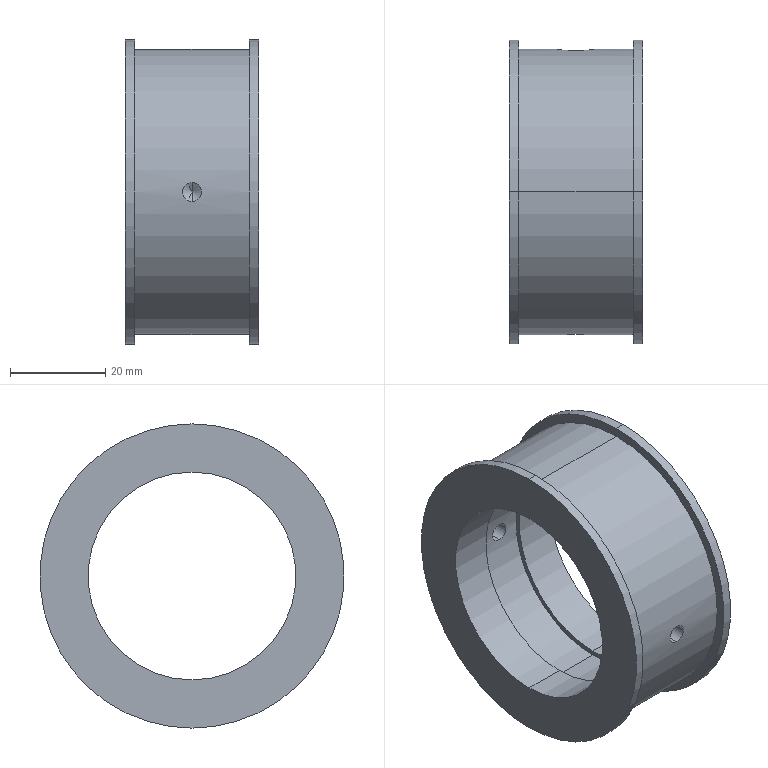Part | SolidWorks | features HoleWzd 3, Fillet 2, Revolution 1 | 1 solid | 31 faces | box 28 x 64 x 64 mm | volume 37136 mm3 | cylinder 18 | plane 7 | torus 2 | spline 2 | cone 2 | commonest cylinder face diameters 4 x4 43.7 x4 64 x4 7.5 x2 45.7 x2 60 x2
STEP:
#1=CARTESIAN_POINT('',(5.61,28.8,3.75));
#2=VERTEX_POINT('',#1);
#3=CARTESIAN_POINT('',(5.61,28.8,-3.75));
#4=VERTEX_POINT('',#3);
#5=CARTESIAN_POINT('',(5.61,28.8,0.));
#6=DIRECTION('',(0.,-1.,0.));
#7=DIRECTION('',(0.,0.,-1.));
#8=AXIS2_PLACEMENT_3D('',#5,#6,#7);
#9=CIRCLE('',#8,3.75);
#10=EDGE_CURVE('',#2,#4,#9,.T.);
#11=ORIENTED_EDGE('',*,*,#10,.F.);
#12=CARTESIAN_POINT('',(5.61,28.5,3.45));
#13=VERTEX_POINT('',#12);
#14=CARTESIAN_POINT('',(5.61,28.8,3.45));
#15=DIRECTION('',(1.,0.,0.));
#16=DIRECTION('',(0.,0.,-1.));
#17=AXIS2_PLACEMENT_3D('',#14,#15,#16);
#18=CIRCLE('',#17,0.3);
#19=EDGE_CURVE('',#2,#13,#18,.T.);
#20=ORIENTED_EDGE('',*,*,#19,.T.);
#21=CARTESIAN_POINT('',(5.61,28.5,-3.45));
#22=VERTEX_POINT('',#21);
#23=CARTESIAN_POINT('',(5.61,28.5,0.));
#24=DIRECTION('',(0.,1.,0.));
#25=DIRECTION('',(0.,0.,-1.));
#26=AXIS2_PLACEMENT_3D('',#23,#24,#25);
#27=CIRCLE('',#26,3.45);
#28=EDGE_CURVE('',#22,#13,#27,.T.);
#29=ORIENTED_EDGE('',*,*,#28,.F.);
#30=CARTESIAN_POINT('',(5.61,28.8,-3.45));
#31=DIRECTION('',(-1.,0.,0.));
#32=DIRECTION('',(0.,0.,1.));
#33=AXIS2_PLACEMENT_3D('',#30,#31,#32);
#34=CIRCLE('',#33,0.3);
#35=EDGE_CURVE('',#4,#22,#34,.T.);
#36=ORIENTED_EDGE('',*,*,#35,.F.);
#37=EDGE_LOOP('',(#11,#20,#29,#36));
#38=FACE_OUTER_BOUND('',#37,.T.);
#39=CARTESIAN_POINT('',(5.61,28.8,0.));
#40=DIRECTION('',(0.,-1.,0.));
#41=DIRECTION('',(0.,0.,-1.));
#42=AXIS2_PLACEMENT_3D('',#39,#40,#41);
#43=TOROIDAL_SURFACE('',#42,3.45,0.3);
#44=ADVANCED_FACE('',(#38),#43,.F.);
#45=CARTESIAN_POINT('',(4.758,29.551,-3.652));
#46=VERTEX_POINT('',#45);
#47=CARTESIAN_POINT('',(5.61,29.537,3.75));
#48=VERTEX_POINT('',#47);
#49=CARTESIAN_POINT('',(4.758,29.551,-3.652));
#50=CARTESIAN_POINT('',(4.535,29.558,-3.6));
#51=CARTESIAN_POINT('',(4.316,29.568,-3.527));
#52=CARTESIAN_POINT('',(3.899,29.591,-3.345));
#53=CARTESIAN_POINT('',(3.701,29.605,-3.236));
#54=CARTESIAN_POINT('',(3.325,29.634,-2.982));
#55=CARTESIAN_POINT('',(3.146,29.65,-2.836));
#56=CARTESIAN_POINT('',(2.822,29.682,-2.518));
#57=CARTESIAN_POINT('',(2.676,29.698,-2.346));
#58=CARTESIAN_POINT('',(2.414,29.728,-1.974));
#59=CARTESIAN_POINT('',(2.299,29.742,-1.774));
#60=CARTESIAN_POINT('',(2.109,29.766,-1.363));
#61=CARTESIAN_POINT('',(2.033,29.776,-1.149));
#62=CARTESIAN_POINT('',(1.92,29.792,-0.7059));
#63=CARTESIAN_POINT('',(1.884,29.797,-0.479));
#64=CARTESIAN_POINT('',(1.854,29.801,-0.02683));
#65=CARTESIAN_POINT('',(1.859,29.8,0.2003));
#66=CARTESIAN_POINT('',(1.911,29.793,0.6567));
#67=CARTESIAN_POINT('',(1.958,29.786,0.8794));
#68=CARTESIAN_POINT('',(2.09,29.769,1.312));
#69=CARTESIAN_POINT('',(2.177,29.757,1.524));
#70=CARTESIAN_POINT('',(2.387,29.731,1.93));
#71=CARTESIAN_POINT('',(2.509,29.717,2.121));
#72=CARTESIAN_POINT('',(2.787,29.686,2.478));
#73=CARTESIAN_POINT('',(2.944,29.67,2.647));
#74=CARTESIAN_POINT('',(3.284,29.638,2.95));
#75=CARTESIAN_POINT('',(3.466,29.623,3.084));
#76=CARTESIAN_POINT('',(3.853,29.594,3.32));
#77=CARTESIAN_POINT('',(4.06,29.581,3.422));
#78=CARTESIAN_POINT('',(4.485,29.56,3.584));
#79=CARTESIAN_POINT('',(4.703,29.552,3.646));
#80=CARTESIAN_POINT('',(5.15,29.54,3.729));
#81=CARTESIAN_POINT('',(5.38,29.537,3.75));
#82=CARTESIAN_POINT('',(5.61,29.537,3.75));
#83=B_SPLINE_CURVE_WITH_KNOTS('',3,(#49,#50,#51,#52,#53,#54,#55,#56,#57,#58,#59,#60,#61,#62,#63,#64,#65,#66,#67,#68,#69,#70,#71,#72,#73,#74,#75,#76,#77,#78,#79,#80,#81,#82),.UNSPECIFIED.,.F.,.F.,(4,2,2,2,2,2,2,2,2,2,2,2,2,2,2,2,4),(0.01269,0.01337,0.01406,0.01474,0.01543,0.01611,0.0168,0.01748,0.01817,0.01885,0.01954,0.02022,0.02091,0.02159,0.02228,0.02296,0.02365),.UNSPECIFIED.);
#84=EDGE_CURVE('',#46,#48,#83,.T.);
#85=ORIENTED_EDGE('',*,*,#84,.F.);
#86=CARTESIAN_POINT('',(4.712,29.749,-3.872));
#87=VERTEX_POINT('',#86);
#88=CARTESIAN_POINT('',(4.712,29.551,-3.847));
#89=DIRECTION('',(-0.9734,0.02959,0.2273));
#90=DIRECTION('',(0.2274,0.,0.9738));
#91=AXIS2_PLACEMENT_3D('',#88,#89,#90);
#92=CIRCLE('',#91,0.2);
#93=EDGE_CURVE('',#46,#87,#92,.T.);
#94=ORIENTED_EDGE('',*,*,#93,.T.);
#95=CARTESIAN_POINT('',(6.509,29.749,3.872));
#96=VERTEX_POINT('',#95);
#97=CARTESIAN_POINT('',(6.509,29.749,3.872));
#98=CARTESIAN_POINT('',(6.254,29.741,3.932));
#99=CARTESIAN_POINT('',(5.996,29.737,3.966));
#100=CARTESIAN_POINT('',(5.474,29.734,3.983));
#101=CARTESIAN_POINT('',(5.21,29.737,3.965));
#102=CARTESIAN_POINT('',(4.698,29.748,3.878));
#103=CARTESIAN_POINT('',(4.449,29.757,3.81));
#104=CARTESIAN_POINT('',(3.965,29.78,3.624));
#105=CARTESIAN_POINT('',(3.729,29.795,3.506));
#106=CARTESIAN_POINT('',(3.293,29.826,3.231));
#107=CARTESIAN_POINT('',(3.089,29.843,3.072));
#108=CARTESIAN_POINT('',(2.711,29.878,2.714));
#109=CARTESIAN_POINT('',(2.541,29.895,2.517));
#110=CARTESIAN_POINT('',(2.244,29.927,2.096));
#111=CARTESIAN_POINT('',(2.114,29.943,1.869));
#112=CARTESIAN_POINT('',(1.902,29.969,1.394));
#113=CARTESIAN_POINT('',(1.82,29.979,1.149));
#114=CARTESIAN_POINT('',(1.704,29.994,0.6447));
#115=CARTESIAN_POINT('',(1.67,29.999,0.3829));
#116=CARTESIAN_POINT('',(1.654,30.001,-0.135));
#117=CARTESIAN_POINT('',(1.671,29.999,-0.3927));
#118=CARTESIAN_POINT('',(1.755,29.987,-0.9056));
#119=CARTESIAN_POINT('',(1.823,29.979,-1.16));
#120=CARTESIAN_POINT('',(2.004,29.956,-1.643));
#121=CARTESIAN_POINT('',(2.118,29.942,-1.876));
#122=CARTESIAN_POINT('',(2.392,29.911,-2.321));
#123=CARTESIAN_POINT('',(2.549,29.894,-2.526));
#124=CARTESIAN_POINT('',(2.9,29.86,-2.904));
#125=CARTESIAN_POINT('',(3.096,29.842,-3.078));
#126=CARTESIAN_POINT('',(3.516,29.809,-3.382));
#127=CARTESIAN_POINT('',(3.739,29.794,-3.512));
#128=CARTESIAN_POINT('',(4.21,29.768,-3.727));
#129=CARTESIAN_POINT('',(4.459,29.757,-3.813));
#130=CARTESIAN_POINT('',(4.712,29.749,-3.872));
#131=B_SPLINE_CURVE_WITH_KNOTS('',3,(#97,#98,#99,#100,#101,#102,#103,#104,#105,#106,#107,#108,#109,#110,#111,#112,#113,#114,#115,#116,#117,#118,#119,#120,#121,#122,#123,#124,#125,#126,#127,#128,#129,#130),.UNSPECIFIED.,.F.,.F.,(4,2,2,2,2,2,2,2,2,2,2,2,2,2,2,2,4),(0.02421,0.025,0.02578,0.02657,0.02735,0.02814,0.02892,0.02971,0.03049,0.03128,0.03206,0.03285,0.03363,0.03442,0.0352,0.03599,0.03677),.UNSPECIFIED.);
#132=EDGE_CURVE('',#96,#87,#131,.T.);
#133=ORIENTED_EDGE('',*,*,#132,.F.);
#134=CARTESIAN_POINT('',(6.463,29.551,3.652));
#135=VERTEX_POINT('',#134);
#136=CARTESIAN_POINT('',(6.509,29.551,3.846));
#137=DIRECTION('',(0.9734,0.02959,-0.2273));
#138=DIRECTION('',(-0.2274,0.,-0.9738));
#139=AXIS2_PLACEMENT_3D('',#136,#137,#138);
#140=CIRCLE('',#139,0.2);
#141=EDGE_CURVE('',#135,#96,#140,.T.);
#142=ORIENTED_EDGE('',*,*,#141,.F.);
#143=CARTESIAN_POINT('',(5.61,29.537,3.75));
#144=CARTESIAN_POINT('',(5.754,29.537,3.75));
#145=CARTESIAN_POINT('',(6.041,29.539,3.733));
#146=CARTESIAN_POINT('',(6.323,29.546,3.684));
#147=CARTESIAN_POINT('',(6.463,29.551,3.652));
#148=B_SPLINE_CURVE_WITH_KNOTS('',3,(#143,#144,#145,#146,#147),.UNSPECIFIED.,.F.,.F.,(4,1,4),(0.,0.0004293,0.0008586),.UNSPECIFIED.);
#149=EDGE_CURVE('',#48,#135,#148,.T.);
#150=ORIENTED_EDGE('',*,*,#149,.F.);
#151=EDGE_LOOP('',(#85,#94,#133,#142,#150));
#152=FACE_OUTER_BOUND('',#151,.T.);
#153=CARTESIAN_POINT('',(6.463,29.551,3.652));
#154=CARTESIAN_POINT('',(6.457,29.778,3.653));
#155=CARTESIAN_POINT('',(6.509,29.749,3.872));
#156=CARTESIAN_POINT('',(6.222,29.543,3.708));
#157=CARTESIAN_POINT('',(6.216,29.771,3.709));
#158=CARTESIAN_POINT('',(6.254,29.741,3.932));
#159=CARTESIAN_POINT('',(5.979,29.538,3.74));
#160=CARTESIAN_POINT('',(5.976,29.767,3.74));
#161=CARTESIAN_POINT('',(5.998,29.737,3.966));
#162=CARTESIAN_POINT('',(5.49,29.536,3.756));
#163=CARTESIAN_POINT('',(5.491,29.765,3.756));
#164=CARTESIAN_POINT('',(5.484,29.734,3.983));
#165=CARTESIAN_POINT('',(5.241,29.539,3.74));
#166=CARTESIAN_POINT('',(5.245,29.767,3.74));
#167=CARTESIAN_POINT('',(5.222,29.737,3.966));
#168=CARTESIAN_POINT('',(4.756,29.55,3.66));
#169=CARTESIAN_POINT('',(4.763,29.777,3.661));
#170=CARTESIAN_POINT('',(4.71,29.748,3.881));
#171=CARTESIAN_POINT('',(4.52,29.558,3.596));
#172=CARTESIAN_POINT('',(4.529,29.784,3.599));
#173=CARTESIAN_POINT('',(4.462,29.757,3.814));
#174=CARTESIAN_POINT('',(4.061,29.581,3.424));
#175=CARTESIAN_POINT('',(4.072,29.804,3.429));
#176=CARTESIAN_POINT('',(3.978,29.78,3.631));
#177=CARTESIAN_POINT('',(3.837,29.595,3.313));
#178=CARTESIAN_POINT('',(3.849,29.817,3.32));
#179=CARTESIAN_POINT('',(3.743,29.794,3.513));
#180=CARTESIAN_POINT('',(3.422,29.626,3.055));
#181=CARTESIAN_POINT('',(3.434,29.844,3.064));
#182=CARTESIAN_POINT('',(3.305,29.825,3.24));
#183=CARTESIAN_POINT('',(3.228,29.643,2.907));
#184=CARTESIAN_POINT('',(3.24,29.859,2.916));
#185=CARTESIAN_POINT('',(3.101,29.842,3.082));
#186=CARTESIAN_POINT('',(2.868,29.677,2.57));
#187=CARTESIAN_POINT('',(2.879,29.89,2.581));
#188=CARTESIAN_POINT('',(2.722,29.877,2.725));
#189=CARTESIAN_POINT('',(2.706,29.695,2.384));
#190=CARTESIAN_POINT('',(2.715,29.905,2.396));
#191=CARTESIAN_POINT('',(2.551,29.894,2.528));
#192=CARTESIAN_POINT('',(2.421,29.727,1.988));
#193=CARTESIAN_POINT('',(2.428,29.934,1.999));
#194=CARTESIAN_POINT('',(2.251,29.927,2.108));
#195=CARTESIAN_POINT('',(2.297,29.742,1.774));
#196=CARTESIAN_POINT('',(2.303,29.948,1.785));
#197=CARTESIAN_POINT('',(2.12,29.942,1.881));
#198=CARTESIAN_POINT('',(2.093,29.768,1.325));
#199=CARTESIAN_POINT('',(2.097,29.971,1.334));
#200=CARTESIAN_POINT('',(1.906,29.968,1.405));
#201=CARTESIAN_POINT('',(2.015,29.779,1.093));
#202=CARTESIAN_POINT('',(2.017,29.981,1.101));
#203=CARTESIAN_POINT('',(1.823,29.979,1.159));
#204=CARTESIAN_POINT('',(1.903,29.794,0.6165));
#205=CARTESIAN_POINT('',(1.904,29.995,0.6213));
#206=CARTESIAN_POINT('',(1.706,29.994,0.6537));
#207=CARTESIAN_POINT('',(1.87,29.799,0.3687));
#208=CARTESIAN_POINT('',(1.871,29.999,0.3714));
#209=CARTESIAN_POINT('',(1.671,29.999,0.391));
#210=CARTESIAN_POINT('',(1.854,29.801,-0.1217));
#211=CARTESIAN_POINT('',(1.854,30.001,-0.1225));
#212=CARTESIAN_POINT('',(1.654,30.001,-0.129));
#213=CARTESIAN_POINT('',(1.87,29.799,-0.3657));
#214=CARTESIAN_POINT('',(1.87,29.999,-0.3686));
#215=CARTESIAN_POINT('',(1.671,29.999,-0.3878));
#216=CARTESIAN_POINT('',(1.95,29.788,-0.8512));
#217=CARTESIAN_POINT('',(1.951,29.989,-0.8574));
#218=CARTESIAN_POINT('',(1.755,29.988,-0.9027));
#219=CARTESIAN_POINT('',(2.014,29.779,-1.092));
#220=CARTESIAN_POINT('',(2.017,29.981,-1.1));
#221=CARTESIAN_POINT('',(1.823,29.979,-1.158));
#222=CARTESIAN_POINT('',(2.187,29.756,-1.549));
#223=CARTESIAN_POINT('',(2.191,29.96,-1.559));
#224=CARTESIAN_POINT('',(2.004,29.956,-1.643));
#225=CARTESIAN_POINT('',(2.295,29.743,-1.769));
#226=CARTESIAN_POINT('',(2.301,29.948,-1.78));
#227=CARTESIAN_POINT('',(2.118,29.942,-1.876));
#228=CARTESIAN_POINT('',(2.556,29.711,-2.189));
#229=CARTESIAN_POINT('',(2.564,29.92,-2.201));
#230=CARTESIAN_POINT('',(2.393,29.911,-2.322));
#231=CARTESIAN_POINT('',(2.705,29.695,-2.383));
#232=CARTESIAN_POINT('',(2.714,29.905,-2.395));
#233=CARTESIAN_POINT('',(2.55,29.894,-2.527));
#234=CARTESIAN_POINT('',(3.038,29.661,-2.74));
#235=CARTESIAN_POINT('',(3.05,29.875,-2.751));
#236=CARTESIAN_POINT('',(2.901,29.86,-2.905));
#237=CARTESIAN_POINT('',(3.225,29.643,-2.904));
#238=CARTESIAN_POINT('',(3.237,29.859,-2.914));
#239=CARTESIAN_POINT('',(3.098,29.842,-3.08));
#240=CARTESIAN_POINT('',(3.624,29.61,-3.19));
#241=CARTESIAN_POINT('',(3.636,29.83,-3.198));
#242=CARTESIAN_POINT('',(3.518,29.809,-3.383));
#243=CARTESIAN_POINT('',(3.835,29.595,-3.312));
#244=CARTESIAN_POINT('',(3.847,29.817,-3.319));
#245=CARTESIAN_POINT('',(3.741,29.794,-3.512));
#246=CARTESIAN_POINT('',(4.282,29.569,-3.515));
#247=CARTESIAN_POINT('',(4.292,29.794,-3.519));
#248=CARTESIAN_POINT('',(4.211,29.768,-3.728));
#249=CARTESIAN_POINT('',(4.518,29.558,-3.596));
#250=CARTESIAN_POINT('',(4.527,29.784,-3.598));
#251=CARTESIAN_POINT('',(4.46,29.757,-3.813));
#252=CARTESIAN_POINT('',(4.758,29.551,-3.652));
#253=CARTESIAN_POINT('',(4.764,29.778,-3.653));
#254=CARTESIAN_POINT('',(4.712,29.749,-3.872));
#255=(BOUNDED_SURFACE()B_SPLINE_SURFACE(3,2,((#153,#154,#155),(#156,#157,#158),(#159,#160,#161),(#162,#163,#164),(#165,#166,#167),(#168,#169,#170),(#171,#172,#173),(#174,#175,#176),(#177,#178,#179),(#180,#181,#182),(#183,#184,#185),(#186,#187,#188),(#189,#190,#191),(#192,#193,#194),(#195,#196,#197),(#198,#199,#200),(#201,#202,#203),(#204,#205,#206),(#207,#208,#209),(#210,#211,#212),(#213,#214,#215),(#216,#217,#218),(#219,#220,#221),(#222,#223,#224),(#225,#226,#227),(#228,#229,#230),(#231,#232,#233),(#234,#235,#236),(#237,#238,#239),(#240,#241,#242),(#243,#244,#245),(#246,#247,#248),(#249,#250,#251),(#252,#253,#254)),.UNSPECIFIED.,.F.,.F.,.F.)B_SPLINE_SURFACE_WITH_KNOTS((4,2,2,2,2,2,2,2,2,2,2,2,2,2,2,2,4),(3,3),(0.,0.0007725,0.001545,0.002318,0.00309,0.003863,0.004635,0.005408,0.00618,0.006953,0.007725,0.008498,0.00927,0.01004,0.01082,0.01159,0.01236),(0.,1.),.UNSPECIFIED.)GEOMETRIC_REPRESENTATION_ITEM()RATIONAL_B_SPLINE_SURFACE(((1.,0.6612,1.),(1.,0.6597,1.),(1.,0.6588,1.),(1.,0.6584,1.),(1.,0.6589,1.),(1.,0.661,1.),(1.,0.6626,1.),(1.,0.6669,1.),(1.,0.6696,1.),(1.,0.6754,1.),(1.,0.6785,1.),(1.,0.6849,1.),(1.,0.688,1.),(1.,0.694,1.),(1.,0.6967,1.),(1.,0.7014,1.),(1.,0.7033,1.),(1.,0.706,1.),(1.,0.7069,1.),(1.,0.7073,1.),(1.,0.7069,1.),(1.,0.7049,1.),(1.,0.7033,1.),(1.,0.6992,1.),(1.,0.6968,1.),(1.,0.6911,1.),(1.,0.688,1.),(1.,0.6817,1.),(1.,0.6785,1.),(1.,0.6724,1.),(1.,0.6696,1.),(1.,0.6647,1.),(1.,0.6626,1.),(1.,0.6612,1.)))REPRESENTATION_ITEM('')SURFACE());
#256=ADVANCED_FACE('',(#152),#255,.T.);
#257=CARTESIAN_POINT('',(5.61,-24.798,0.));
#258=VERTEX_POINT('',#257);
#259=CARTESIAN_POINT('',(5.61,-26.,-2.));
#260=VERTEX_POINT('',#259);
#261=CARTESIAN_POINT('',(5.61,-26.,-2.));
#262=DIRECTION('',(0.,-0.515,-0.8572));
#263=VECTOR('',#262,1000.);
#264=LINE('',#261,#263);
#265=EDGE_CURVE('',#258,#260,#264,.T.);
#266=ORIENTED_EDGE('',*,*,#265,.F.);
#267=CARTESIAN_POINT('',(5.61,-26.,2.));
#268=VERTEX_POINT('',#267);
#269=CARTESIAN_POINT('',(5.61,-26.,2.));
#270=DIRECTION('',(0.,-0.515,0.8572));
#271=VECTOR('',#270,1000.);
#272=LINE('',#269,#271);
#273=EDGE_CURVE('',#258,#268,#272,.T.);
#274=ORIENTED_EDGE('',*,*,#273,.T.);
#275=CARTESIAN_POINT('',(5.61,-26.,0.));
#276=DIRECTION('',(0.,-1.,0.));
#277=DIRECTION('',(0.,0.,-1.));
#278=AXIS2_PLACEMENT_3D('',#275,#276,#277);
#279=CIRCLE('',#278,2.);
#280=EDGE_CURVE('',#268,#260,#279,.T.);
#281=ORIENTED_EDGE('',*,*,#280,.T.);
#282=EDGE_LOOP('',(#266,#274,#281));
#283=FACE_OUTER_BOUND('',#282,.T.);
#284=CARTESIAN_POINT('',(5.61,-26.,0.));
#285=DIRECTION('',(0.,-1.,0.));
#286=DIRECTION('',(0.,0.,-1.));
#287=AXIS2_PLACEMENT_3D('',#284,#285,#286);
#288=CONICAL_SURFACE('',#287,2.,1.03);
#289=ADVANCED_FACE('',(#283),#288,.F.);
#290=ORIENTED_EDGE('',*,*,#280,.F.);
#291=CARTESIAN_POINT('',(5.61,-29.933,2.));
#292=VERTEX_POINT('',#291);
#293=CARTESIAN_POINT('',(5.61,-30.,2.));
#294=DIRECTION('',(0.,-1.,0.));
#295=VECTOR('',#294,1000.);
#296=LINE('',#293,#295);
#297=EDGE_CURVE('',#268,#292,#296,.T.);
#298=ORIENTED_EDGE('',*,*,#297,.T.);
#299=CARTESIAN_POINT('',(5.61,-29.933,-2.));
#300=VERTEX_POINT('',#299);
#301=CARTESIAN_POINT('',(5.61,-29.933,-2.));
#302=CARTESIAN_POINT('',(5.478,-29.933,-2.));
#303=CARTESIAN_POINT('',(5.348,-29.934,-1.987));
#304=CARTESIAN_POINT('',(5.093,-29.937,-1.936));
#305=CARTESIAN_POINT('',(4.965,-29.94,-1.898));
#306=CARTESIAN_POINT('',(4.723,-29.946,-1.797));
#307=CARTESIAN_POINT('',(4.608,-29.95,-1.736));
#308=CARTESIAN_POINT('',(4.391,-29.958,-1.591));
#309=CARTESIAN_POINT('',(4.288,-29.962,-1.506));
#310=CARTESIAN_POINT('',(4.011,-29.975,-1.229));
#311=CARTESIAN_POINT('',(3.862,-29.984,-1.006));
#312=CARTESIAN_POINT('',(3.663,-29.996,-0.525));
#313=CARTESIAN_POINT('',(3.61,-30.,-0.2617));
#314=CARTESIAN_POINT('',(3.61,-30.,0.1298));
#315=CARTESIAN_POINT('',(3.623,-29.999,0.2623));
#316=CARTESIAN_POINT('',(3.674,-29.996,0.5189));
#317=CARTESIAN_POINT('',(3.712,-29.993,0.6436));
#318=CARTESIAN_POINT('',(3.812,-29.987,0.8858));
#319=CARTESIAN_POINT('',(3.875,-29.983,1.003));
#320=CARTESIAN_POINT('',(4.02,-29.975,1.22));
#321=CARTESIAN_POINT('',(4.102,-29.971,1.321));
#322=CARTESIAN_POINT('',(4.289,-29.962,1.507));
#323=CARTESIAN_POINT('',(4.39,-29.958,1.59));
#324=CARTESIAN_POINT('',(4.607,-29.95,1.735));
#325=CARTESIAN_POINT('',(4.724,-29.946,1.798));
#326=CARTESIAN_POINT('',(4.966,-29.94,1.898));
#327=CARTESIAN_POINT('',(5.091,-29.937,1.936));
#328=CARTESIAN_POINT('',(5.347,-29.934,1.987));
#329=CARTESIAN_POINT('',(5.48,-29.933,2.));
#330=CARTESIAN_POINT('',(5.61,-29.933,2.));
#331=B_SPLINE_CURVE_WITH_KNOTS('',3,(#301,#302,#303,#304,#305,#306,#307,#308,#309,#310,#311,#312,#313,#314,#315,#316,#317,#318,#319,#320,#321,#322,#323,#324,#325,#326,#327,#328,#329,#330),.UNSPECIFIED.,.F.,.F.,(4,2,2,2,2,2,2,2,2,2,2,2,2,2,4),(0.,0.0003909,0.0007818,0.001173,0.001564,0.002345,0.003127,0.003518,0.003909,0.0043,0.004691,0.005082,0.005473,0.005864,0.006255),.UNSPECIFIED.);
#332=EDGE_CURVE('',#300,#292,#331,.T.);
#333=ORIENTED_EDGE('',*,*,#332,.F.);
#334=CARTESIAN_POINT('',(5.61,-30.,-2.));
#335=DIRECTION('',(0.,-1.,0.));
#336=VECTOR('',#335,1000.);
#337=LINE('',#334,#336);
#338=EDGE_CURVE('',#260,#300,#337,.T.);
#339=ORIENTED_EDGE('',*,*,#338,.F.);
#340=EDGE_LOOP('',(#290,#298,#333,#339));
#341=FACE_OUTER_BOUND('',#340,.T.);
#342=CARTESIAN_POINT('',(5.61,-30.,0.));
#343=DIRECTION('',(0.,-1.,0.));
#344=DIRECTION('',(0.,0.,-1.));
#345=AXIS2_PLACEMENT_3D('',#342,#343,#344);
#346=CYLINDRICAL_SURFACE('',#345,2.);
#347=ADVANCED_FACE('',(#341),#346,.F.);
#348=CARTESIAN_POINT('',(5.61,22.762,-2.));
#349=VERTEX_POINT('',#348);
#350=CARTESIAN_POINT('',(5.61,22.762,2.));
#351=VERTEX_POINT('',#350);
#352=CARTESIAN_POINT('',(5.61,22.762,-2.));
#353=CARTESIAN_POINT('',(5.349,22.762,-2.));
#354=CARTESIAN_POINT('',(5.086,22.767,-1.948));
#355=CARTESIAN_POINT('',(4.605,22.783,-1.748));
#356=CARTESIAN_POINT('',(4.382,22.795,-1.599));
#357=CARTESIAN_POINT('',(4.105,22.812,-1.323));
#358=CARTESIAN_POINT('',(4.02,22.818,-1.22));
#359=CARTESIAN_POINT('',(3.875,22.828,-1.003));
#360=CARTESIAN_POINT('',(3.814,22.833,-0.8882));
#361=CARTESIAN_POINT('',(3.713,22.841,-0.6463));
#362=CARTESIAN_POINT('',(3.675,22.844,-0.5192));
#363=CARTESIAN_POINT('',(3.623,22.849,-0.2635));
#364=CARTESIAN_POINT('',(3.61,22.85,-0.1336));
#365=CARTESIAN_POINT('',(3.61,22.85,0.1305));
#366=CARTESIAN_POINT('',(3.623,22.849,0.2608));
#367=CARTESIAN_POINT('',(3.674,22.845,0.5164));
#368=CARTESIAN_POINT('',(3.712,22.841,0.6434));
#369=CARTESIAN_POINT('',(3.812,22.833,0.8857));
#370=CARTESIAN_POINT('',(3.874,22.828,1.001));
#371=CARTESIAN_POINT('',(4.019,22.818,1.218));
#372=CARTESIAN_POINT('',(4.103,22.812,1.321));
#373=CARTESIAN_POINT('',(4.379,22.795,1.598));
#374=CARTESIAN_POINT('',(4.602,22.783,1.747));
#375=CARTESIAN_POINT('',(5.083,22.767,1.947));
#376=CARTESIAN_POINT('',(5.346,22.762,2.));
#377=CARTESIAN_POINT('',(5.61,22.762,2.));
#378=B_SPLINE_CURVE_WITH_KNOTS('',3,(#352,#353,#354,#355,#356,#357,#358,#359,#360,#361,#362,#363,#364,#365,#366,#367,#368,#369,#370,#371,#372,#373,#374,#375,#376,#377),.UNSPECIFIED.,.F.,.F.,(4,2,2,2,2,2,2,2,2,2,2,2,4),(0.006256,0.007038,0.00782,0.00821,0.008601,0.008992,0.009383,0.009774,0.01016,0.01056,0.01095,0.01173,0.01251),.UNSPECIFIED.);
#379=EDGE_CURVE('',#349,#351,#378,.T.);
#380=ORIENTED_EDGE('',*,*,#379,.F.);
#381=CARTESIAN_POINT('',(5.61,28.5,-2.));
#382=VERTEX_POINT('',#381);
#383=CARTESIAN_POINT('',(5.61,28.5,-2.));
#384=DIRECTION('',(0.,1.,0.));
#385=VECTOR('',#384,1000.);
#386=LINE('',#383,#385);
#387=EDGE_CURVE('',#349,#382,#386,.T.);
#388=ORIENTED_EDGE('',*,*,#387,.T.);
#389=CARTESIAN_POINT('',(5.61,28.5,2.));
#390=VERTEX_POINT('',#389);
#391=CARTESIAN_POINT('',(5.61,28.5,0.));
#392=DIRECTION('',(0.,1.,0.));
#393=DIRECTION('',(0.,0.,1.));
#394=AXIS2_PLACEMENT_3D('',#391,#392,#393);
#395=CIRCLE('',#394,2.);
#396=EDGE_CURVE('',#382,#390,#395,.T.);
#397=ORIENTED_EDGE('',*,*,#396,.T.);
#398=CARTESIAN_POINT('',(5.61,28.5,2.));
#399=DIRECTION('',(0.,1.,0.));
#400=VECTOR('',#399,1000.);
#401=LINE('',#398,#400);
#402=EDGE_CURVE('',#351,#390,#401,.T.);
#403=ORIENTED_EDGE('',*,*,#402,.F.);
#404=EDGE_LOOP('',(#380,#388,#397,#403));
#405=FACE_OUTER_BOUND('',#404,.T.);
#406=CARTESIAN_POINT('',(5.61,28.5,0.));
#407=DIRECTION('',(0.,1.,0.));
#408=DIRECTION('',(0.,0.,1.));
#409=AXIS2_PLACEMENT_3D('',#406,#407,#408);
#410=CYLINDRICAL_SURFACE('',#409,2.);
#411=ADVANCED_FACE('',(#405),#410,.F.);
#412=ORIENTED_EDGE('',*,*,#10,.T.);
#413=CARTESIAN_POINT('',(5.61,29.537,-3.75));
#414=VERTEX_POINT('',#413);
#415=CARTESIAN_POINT('',(5.61,30.,-3.75));
#416=DIRECTION('',(0.,1.,0.));
#417=VECTOR('',#416,1000.);
#418=LINE('',#415,#417);
#419=EDGE_CURVE('',#4,#414,#418,.T.);
#420=ORIENTED_EDGE('',*,*,#419,.T.);
#421=CARTESIAN_POINT('',(5.61,29.537,-3.75));
#422=CARTESIAN_POINT('',(5.468,29.537,-3.75));
#423=CARTESIAN_POINT('',(5.325,29.538,-3.742));
#424=CARTESIAN_POINT('',(5.038,29.543,-3.709));
#425=CARTESIAN_POINT('',(4.897,29.546,-3.684));
#426=CARTESIAN_POINT('',(4.758,29.551,-3.652));
#427=B_SPLINE_CURVE_WITH_KNOTS('',3,(#421,#422,#423,#424,#425,#426),.UNSPECIFIED.,.F.,.F.,(4,2,4),(0.01183,0.01226,0.01269),.UNSPECIFIED.);
#428=EDGE_CURVE('',#414,#46,#427,.T.);
#429=ORIENTED_EDGE('',*,*,#428,.T.);
#430=ORIENTED_EDGE('',*,*,#84,.T.);
#431=CARTESIAN_POINT('',(5.61,30.,3.75));
#432=DIRECTION('',(0.,1.,0.));
#433=VECTOR('',#432,1000.);
#434=LINE('',#431,#433);
#435=EDGE_CURVE('',#2,#48,#434,.T.);
#436=ORIENTED_EDGE('',*,*,#435,.F.);
#437=EDGE_LOOP('',(#412,#420,#429,#430,#436));
#438=FACE_OUTER_BOUND('',#437,.T.);
#439=CARTESIAN_POINT('',(5.61,30.,0.));
#440=DIRECTION('',(0.,1.,0.));
#441=DIRECTION('',(0.,0.,1.));
#442=AXIS2_PLACEMENT_3D('',#439,#440,#441);
#443=CYLINDRICAL_SURFACE('',#442,3.75);
#444=ADVANCED_FACE('',(#438),#443,.F.);
#445=CARTESIAN_POINT('',(0.6103,0.,-21.85));
#446=VERTEX_POINT('',#445);
#447=CARTESIAN_POINT('',(0.6103,0.,21.85));
#448=VERTEX_POINT('',#447);
#449=CARTESIAN_POINT('',(0.6103,0.,0.));
#450=DIRECTION('',(-1.,0.,0.));
#451=DIRECTION('',(0.,0.,1.));
#452=AXIS2_PLACEMENT_3D('',#449,#450,#451);
#453=CIRCLE('',#452,21.85);
#454=EDGE_CURVE('',#446,#448,#453,.T.);
#455=ORIENTED_EDGE('',*,*,#454,.F.);
#456=CARTESIAN_POINT('',(-8.39,0.,-21.85));
#457=VERTEX_POINT('',#456);
#458=CARTESIAN_POINT('',(-19.037,0.,-21.85));
#459=DIRECTION('',(-1.,0.,0.));
#460=VECTOR('',#459,1000.);
#461=LINE('',#458,#460);
#462=EDGE_CURVE('',#446,#457,#461,.T.);
#463=ORIENTED_EDGE('',*,*,#462,.T.);
#464=CARTESIAN_POINT('',(-8.39,0.,21.85));
#465=VERTEX_POINT('',#464);
#466=CARTESIAN_POINT('',(-8.39,0.,0.));
#467=DIRECTION('',(-1.,0.,0.));
#468=DIRECTION('',(0.,0.,1.));
#469=AXIS2_PLACEMENT_3D('',#466,#467,#468);
#470=CIRCLE('',#469,21.85);
#471=EDGE_CURVE('',#457,#465,#470,.T.);
#472=ORIENTED_EDGE('',*,*,#471,.T.);
#473=CARTESIAN_POINT('',(-19.037,0.,21.85));
#474=DIRECTION('',(-1.,0.,0.));
#475=VECTOR('',#474,1000.);
#476=LINE('',#473,#475);
#477=EDGE_CURVE('',#448,#465,#476,.T.);
#478=ORIENTED_EDGE('',*,*,#477,.F.);
#479=EDGE_LOOP('',(#455,#463,#472,#478));
#480=FACE_OUTER_BOUND('',#479,.T.);
#481=CARTESIAN_POINT('',(-19.037,0.,0.));
#482=DIRECTION('',(-1.,0.,0.));
#483=DIRECTION('',(0.,0.,1.));
#484=AXIS2_PLACEMENT_3D('',#481,#482,#483);
#485=CYLINDRICAL_SURFACE('',#484,21.85);
#486=ADVANCED_FACE('',(#480),#485,.F.);
#487=CARTESIAN_POINT('',(10.61,0.,-22.85));
#488=VERTEX_POINT('',#487);
#489=CARTESIAN_POINT('',(10.61,0.,22.85));
#490=VERTEX_POINT('',#489);
#491=CARTESIAN_POINT('',(10.61,0.,0.));
#492=DIRECTION('',(-1.,0.,0.));
#493=DIRECTION('',(0.,0.,1.));
#494=AXIS2_PLACEMENT_3D('',#491,#492,#493);
#495=CIRCLE('',#494,22.85);
#496=EDGE_CURVE('',#488,#490,#495,.T.);
#497=ORIENTED_EDGE('',*,*,#496,.F.);
#498=CARTESIAN_POINT('',(0.6103,0.,-22.85));
#499=VERTEX_POINT('',#498);
#500=CARTESIAN_POINT('',(-19.037,0.,-22.85));
#501=DIRECTION('',(-1.,0.,0.));
#502=VECTOR('',#501,1000.);
#503=LINE('',#500,#502);
#504=EDGE_CURVE('',#488,#499,#503,.T.);
#505=ORIENTED_EDGE('',*,*,#504,.T.);
#506=CARTESIAN_POINT('',(0.6103,0.,22.85));
#507=VERTEX_POINT('',#506);
#508=CARTESIAN_POINT('',(0.6103,0.,0.));
#509=DIRECTION('',(-1.,0.,0.));
#510=DIRECTION('',(0.,0.,1.));
#511=AXIS2_PLACEMENT_3D('',#508,#509,#510);
#512=CIRCLE('',#511,22.85);
#513=EDGE_CURVE('',#499,#507,#512,.T.);
#514=ORIENTED_EDGE('',*,*,#513,.T.);
#515=CARTESIAN_POINT('',(-19.037,0.,22.85));
#516=DIRECTION('',(-1.,0.,0.));
#517=VECTOR('',#516,1000.);
#518=LINE('',#515,#517);
#519=EDGE_CURVE('',#490,#507,#518,.T.);
#520=ORIENTED_EDGE('',*,*,#519,.F.);
#521=EDGE_LOOP('',(#497,#505,#514,#520));
#522=FACE_OUTER_BOUND('',#521,.T.);
#523=CARTESIAN_POINT('',(-19.037,0.,0.));
#524=DIRECTION('',(-1.,0.,0.));
#525=DIRECTION('',(0.,0.,1.));
#526=AXIS2_PLACEMENT_3D('',#523,#524,#525);
#527=CYLINDRICAL_SURFACE('',#526,22.85);
#528=ADVANCED_FACE('',(#522),#527,.F.);
#529=CARTESIAN_POINT('',(19.61,0.,-21.85));
#530=VERTEX_POINT('',#529);
#531=CARTESIAN_POINT('',(19.61,0.,21.85));
#532=VERTEX_POINT('',#531);
#533=CARTESIAN_POINT('',(19.61,0.,0.));
#534=DIRECTION('',(-1.,0.,0.));
#535=DIRECTION('',(0.,0.,1.));
#536=AXIS2_PLACEMENT_3D('',#533,#534,#535);
#537=CIRCLE('',#536,21.85);
#538=EDGE_CURVE('',#530,#532,#537,.T.);
#539=ORIENTED_EDGE('',*,*,#538,.F.);
#540=CARTESIAN_POINT('',(10.61,0.,-21.85));
#541=VERTEX_POINT('',#540);
#542=CARTESIAN_POINT('',(-19.037,0.,-21.85));
#543=DIRECTION('',(-1.,0.,0.));
#544=VECTOR('',#543,1000.);
#545=LINE('',#542,#544);
#546=EDGE_CURVE('',#530,#541,#545,.T.);
#547=ORIENTED_EDGE('',*,*,#546,.T.);
#548=CARTESIAN_POINT('',(10.61,0.,21.85));
#549=VERTEX_POINT('',#548);
#550=CARTESIAN_POINT('',(10.61,0.,0.));
#551=DIRECTION('',(-1.,0.,0.));
#552=DIRECTION('',(0.,0.,1.));
#553=AXIS2_PLACEMENT_3D('',#550,#551,#552);
#554=CIRCLE('',#553,21.85);
#555=EDGE_CURVE('',#541,#549,#554,.T.);
#556=ORIENTED_EDGE('',*,*,#555,.T.);
#557=CARTESIAN_POINT('',(-19.037,0.,21.85));
#558=DIRECTION('',(-1.,0.,0.));
#559=VECTOR('',#558,1000.);
#560=LINE('',#557,#559);
#561=EDGE_CURVE('',#532,#549,#560,.T.);
#562=ORIENTED_EDGE('',*,*,#561,.F.);
#563=EDGE_LOOP('',(#539,#547,#556,#562));
#564=FACE_OUTER_BOUND('',#563,.T.);
#565=CARTESIAN_POINT('',(-19.037,0.,0.));
#566=DIRECTION('',(-1.,0.,0.));
#567=DIRECTION('',(0.,0.,1.));
#568=AXIS2_PLACEMENT_3D('',#565,#566,#567);
#569=CYLINDRICAL_SURFACE('',#568,21.85);
#570=ADVANCED_FACE('',(#564),#569,.F.);
#571=CARTESIAN_POINT('',(19.61,0.,32.));
#572=VERTEX_POINT('',#571);
#573=CARTESIAN_POINT('',(19.61,0.,-32.));
#574=VERTEX_POINT('',#573);
#575=CARTESIAN_POINT('',(19.61,0.,0.));
#576=DIRECTION('',(-1.,0.,0.));
#577=DIRECTION('',(0.,0.,1.));
#578=AXIS2_PLACEMENT_3D('',#575,#576,#577);
#579=CIRCLE('',#578,32.);
#580=EDGE_CURVE('',#572,#574,#579,.T.);
#581=ORIENTED_EDGE('',*,*,#580,.T.);
#582=CARTESIAN_POINT('',(17.61,0.,-32.));
#583=VERTEX_POINT('',#582);
#584=CARTESIAN_POINT('',(-19.037,0.,-32.));
#585=DIRECTION('',(-1.,0.,0.));
#586=VECTOR('',#585,1000.);
#587=LINE('',#584,#586);
#588=EDGE_CURVE('',#574,#583,#587,.T.);
#589=ORIENTED_EDGE('',*,*,#588,.T.);
#590=CARTESIAN_POINT('',(17.61,0.,32.));
#591=VERTEX_POINT('',#590);
#592=CARTESIAN_POINT('',(17.61,0.,0.));
#593=DIRECTION('',(-1.,0.,0.));
#594=DIRECTION('',(0.,0.,1.));
#595=AXIS2_PLACEMENT_3D('',#592,#593,#594);
#596=CIRCLE('',#595,32.);
#597=EDGE_CURVE('',#591,#583,#596,.T.);
#598=ORIENTED_EDGE('',*,*,#597,.F.);
#599=CARTESIAN_POINT('',(-19.037,0.,32.));
#600=DIRECTION('',(-1.,0.,0.));
#601=VECTOR('',#600,1000.);
#602=LINE('',#599,#601);
#603=EDGE_CURVE('',#572,#591,#602,.T.);
#604=ORIENTED_EDGE('',*,*,#603,.F.);
#605=EDGE_LOOP('',(#581,#589,#598,#604));
#606=FACE_OUTER_BOUND('',#605,.T.);
#607=CARTESIAN_POINT('',(-19.037,0.,0.));
#608=DIRECTION('',(-1.,0.,0.));
#609=DIRECTION('',(0.,0.,1.));
#610=AXIS2_PLACEMENT_3D('',#607,#608,#609);
#611=CYLINDRICAL_SURFACE('',#610,32.);
#612=ADVANCED_FACE('',(#606),#611,.T.);
#613=ORIENTED_EDGE('',*,*,#132,.T.);
#614=CARTESIAN_POINT('',(4.712,29.749,-3.872));
#615=CARTESIAN_POINT('',(4.965,29.741,-3.932));
#616=CARTESIAN_POINT('',(5.227,29.737,-3.966));
#617=CARTESIAN_POINT('',(5.746,29.734,-3.983));
#618=CARTESIAN_POINT('',(6.003,29.737,-3.965));
#619=CARTESIAN_POINT('',(6.516,29.748,-3.879));
#620=CARTESIAN_POINT('',(6.77,29.757,-3.81));
#621=CARTESIAN_POINT('',(7.253,29.78,-3.626));
#622=CARTESIAN_POINT('',(7.484,29.794,-3.51));
#623=CARTESIAN_POINT('',(7.927,29.826,-3.232));
#624=CARTESIAN_POINT('',(8.131,29.843,-3.073));
#625=CARTESIAN_POINT('',(8.505,29.877,-2.718));
#626=CARTESIAN_POINT('',(8.677,29.895,-2.519));
#627=CARTESIAN_POINT('',(8.977,29.927,-2.096));
#628=CARTESIAN_POINT('',(9.105,29.942,-1.872));
#629=CARTESIAN_POINT('',(9.317,29.968,-1.399));
#630=CARTESIAN_POINT('',(9.401,29.979,-1.149));
#631=CARTESIAN_POINT('',(9.517,29.994,-0.6445));
#632=CARTESIAN_POINT('',(9.55,29.999,-0.3881));
#633=CARTESIAN_POINT('',(9.567,30.001,0.1335));
#634=CARTESIAN_POINT('',(9.549,29.998,0.3946));
#635=CARTESIAN_POINT('',(9.465,29.987,0.9045));
#636=CARTESIAN_POINT('',(9.398,29.979,1.157));
#637=CARTESIAN_POINT('',(9.216,29.956,1.646));
#638=CARTESIAN_POINT('',(9.102,29.942,1.877));
#639=CARTESIAN_POINT('',(8.831,29.911,2.317));
#640=CARTESIAN_POINT('',(8.671,29.894,2.527));
#641=CARTESIAN_POINT('',(8.319,29.86,2.906));
#642=CARTESIAN_POINT('',(8.126,29.842,3.077));
#643=CARTESIAN_POINT('',(7.705,29.809,3.381));
#644=CARTESIAN_POINT('',(7.478,29.794,3.514));
#645=CARTESIAN_POINT('',(7.008,29.768,3.728));
#646=CARTESIAN_POINT('',(6.764,29.757,3.812));
#647=CARTESIAN_POINT('',(6.509,29.749,3.872));
#648=B_SPLINE_CURVE_WITH_KNOTS('',3,(#614,#615,#616,#617,#618,#619,#620,#621,#622,#623,#624,#625,#626,#627,#628,#629,#630,#631,#632,#633,#634,#635,#636,#637,#638,#639,#640,#641,#642,#643,#644,#645,#646,#647),.UNSPECIFIED.,.F.,.F.,(4,2,2,2,2,2,2,2,2,2,2,2,2,2,2,2,4),(0.01165,0.01243,0.01322,0.014,0.01479,0.01557,0.01636,0.01714,0.01793,0.01872,0.0195,0.02029,0.02107,0.02186,0.02264,0.02343,0.02421),.UNSPECIFIED.);
#649=EDGE_CURVE('',#87,#96,#648,.T.);
#650=ORIENTED_EDGE('',*,*,#649,.T.);
#651=EDGE_LOOP('',(#613,#650));
#652=FACE_BOUND('',#651,.T.);
#653=CARTESIAN_POINT('',(17.61,0.,30.));
#654=VERTEX_POINT('',#653);
#655=CARTESIAN_POINT('',(17.61,0.,-30.));
#656=VERTEX_POINT('',#655);
#657=CARTESIAN_POINT('',(17.61,0.,0.));
#658=DIRECTION('',(-1.,0.,0.));
#659=DIRECTION('',(0.,0.,1.));
#660=AXIS2_PLACEMENT_3D('',#657,#658,#659);
#661=CIRCLE('',#660,30.);
#662=EDGE_CURVE('',#654,#656,#661,.T.);
#663=ORIENTED_EDGE('',*,*,#662,.T.);
#664=CARTESIAN_POINT('',(-6.39,0.,-30.));
#665=VERTEX_POINT('',#664);
#666=CARTESIAN_POINT('',(-19.037,0.,-30.));
#667=DIRECTION('',(-1.,0.,0.));
#668=VECTOR('',#667,1000.);
#669=LINE('',#666,#668);
#670=EDGE_CURVE('',#656,#665,#669,.T.);
#671=ORIENTED_EDGE('',*,*,#670,.T.);
#672=CARTESIAN_POINT('',(-6.39,0.,30.));
#673=VERTEX_POINT('',#672);
#674=CARTESIAN_POINT('',(-6.39,0.,0.));
#675=DIRECTION('',(-1.,0.,0.));
#676=DIRECTION('',(0.,0.,1.));
#677=AXIS2_PLACEMENT_3D('',#674,#675,#676);
#678=CIRCLE('',#677,30.);
#679=EDGE_CURVE('',#673,#665,#678,.T.);
#680=ORIENTED_EDGE('',*,*,#679,.F.);
#681=CARTESIAN_POINT('',(-19.037,0.,30.));
#682=DIRECTION('',(-1.,0.,0.));
#683=VECTOR('',#682,1000.);
#684=LINE('',#681,#683);
#685=EDGE_CURVE('',#654,#673,#684,.T.);
#686=ORIENTED_EDGE('',*,*,#685,.F.);
#687=EDGE_LOOP('',(#663,#671,#680,#686));
#688=FACE_OUTER_BOUND('',#687,.T.);
#689=CARTESIAN_POINT('',(-19.037,0.,0.));
#690=DIRECTION('',(-1.,0.,0.));
#691=DIRECTION('',(0.,0.,1.));
#692=AXIS2_PLACEMENT_3D('',#689,#690,#691);
#693=CYLINDRICAL_SURFACE('',#692,30.);
#694=ADVANCED_FACE('',(#652,#688),#693,.T.);
#695=CARTESIAN_POINT('',(-6.39,0.,32.));
#696=VERTEX_POINT('',#695);
#697=CARTESIAN_POINT('',(-6.39,0.,-32.));
#698=VERTEX_POINT('',#697);
#699=CARTESIAN_POINT('',(-6.39,0.,0.));
#700=DIRECTION('',(-1.,0.,0.));
#701=DIRECTION('',(0.,0.,1.));
#702=AXIS2_PLACEMENT_3D('',#699,#700,#701);
#703=CIRCLE('',#702,32.);
#704=EDGE_CURVE('',#696,#698,#703,.T.);
#705=ORIENTED_EDGE('',*,*,#704,.T.);
#706=CARTESIAN_POINT('',(-8.39,0.,-32.));
#707=VERTEX_POINT('',#706);
#708=CARTESIAN_POINT('',(-19.037,0.,-32.));
#709=DIRECTION('',(-1.,0.,0.));
#710=VECTOR('',#709,1000.);
#711=LINE('',#708,#710);
#712=EDGE_CURVE('',#698,#707,#711,.T.);
#713=ORIENTED_EDGE('',*,*,#712,.T.);
#714=CARTESIAN_POINT('',(-8.39,0.,32.));
#715=VERTEX_POINT('',#714);
#716=CARTESIAN_POINT('',(-8.39,0.,0.));
#717=DIRECTION('',(-1.,0.,0.));
#718=DIRECTION('',(0.,0.,1.));
#719=AXIS2_PLACEMENT_3D('',#716,#717,#718);
#720=CIRCLE('',#719,32.);
#721=EDGE_CURVE('',#715,#707,#720,.T.);
#722=ORIENTED_EDGE('',*,*,#721,.F.);
#723=CARTESIAN_POINT('',(-19.037,0.,32.));
#724=DIRECTION('',(-1.,0.,0.));
#725=VECTOR('',#724,1000.);
#726=LINE('',#723,#725);
#727=EDGE_CURVE('',#696,#715,#726,.T.);
#728=ORIENTED_EDGE('',*,*,#727,.F.);
#729=EDGE_LOOP('',(#705,#713,#722,#728));
#730=FACE_OUTER_BOUND('',#729,.T.);
#731=CARTESIAN_POINT('',(-19.037,0.,0.));
#732=DIRECTION('',(-1.,0.,0.));
#733=DIRECTION('',(0.,0.,1.));
#734=AXIS2_PLACEMENT_3D('',#731,#732,#733);
#735=CYLINDRICAL_SURFACE('',#734,32.);
#736=ADVANCED_FACE('',(#730),#735,.T.);
#737=ORIENTED_EDGE('',*,*,#712,.F.);
#738=CARTESIAN_POINT('',(-6.39,0.,0.));
#739=DIRECTION('',(-1.,0.,0.));
#740=DIRECTION('',(0.,0.,1.));
#741=AXIS2_PLACEMENT_3D('',#738,#739,#740);
#742=CIRCLE('',#741,32.);
#743=EDGE_CURVE('',#698,#696,#742,.T.);
#744=ORIENTED_EDGE('',*,*,#743,.T.);
#745=ORIENTED_EDGE('',*,*,#727,.T.);
#746=CARTESIAN_POINT('',(-8.39,0.,0.));
#747=DIRECTION('',(-1.,0.,0.));
#748=DIRECTION('',(0.,0.,1.));
#749=AXIS2_PLACEMENT_3D('',#746,#747,#748);
#750=CIRCLE('',#749,32.);
#751=EDGE_CURVE('',#707,#715,#750,.T.);
#752=ORIENTED_EDGE('',*,*,#751,.F.);
#753=EDGE_LOOP('',(#737,#744,#745,#752));
#754=FACE_OUTER_BOUND('',#753,.T.);
#755=CARTESIAN_POINT('',(-19.037,0.,0.));
#756=DIRECTION('',(-1.,0.,0.));
#757=DIRECTION('',(0.,0.,1.));
#758=AXIS2_PLACEMENT_3D('',#755,#756,#757);
#759=CYLINDRICAL_SURFACE('',#758,32.);
#760=ADVANCED_FACE('',(#754),#759,.T.);
#761=ORIENTED_EDGE('',*,*,#704,.F.);
#762=ORIENTED_EDGE('',*,*,#743,.F.);
#763=EDGE_LOOP('',(#761,#762));
#764=FACE_OUTER_BOUND('',#763,.T.);
#765=ORIENTED_EDGE('',*,*,#679,.T.);
#766=CARTESIAN_POINT('',(-6.39,0.,0.));
#767=DIRECTION('',(-1.,0.,0.));
#768=DIRECTION('',(0.,0.,1.));
#769=AXIS2_PLACEMENT_3D('',#766,#767,#768);
#770=CIRCLE('',#769,30.);
#771=EDGE_CURVE('',#665,#673,#770,.T.);
#772=ORIENTED_EDGE('',*,*,#771,.T.);
#773=EDGE_LOOP('',(#765,#772));
#774=FACE_BOUND('',#773,.T.);
#775=CARTESIAN_POINT('',(-6.39,32.,0.));
#776=DIRECTION('',(-1.,0.,0.));
#777=DIRECTION('',(0.,0.,1.));
#778=AXIS2_PLACEMENT_3D('',#775,#776,#777);
#779=PLANE('',#778);
#780=ADVANCED_FACE('',(#764,#774),#779,.F.);
#781=ORIENTED_EDGE('',*,*,#670,.F.);
#782=CARTESIAN_POINT('',(17.61,0.,0.));
#783=DIRECTION('',(-1.,0.,0.));
#784=DIRECTION('',(0.,0.,1.));
#785=AXIS2_PLACEMENT_3D('',#782,#783,#784);
#786=CIRCLE('',#785,30.);
#787=EDGE_CURVE('',#656,#654,#786,.T.);
#788=ORIENTED_EDGE('',*,*,#787,.T.);
#789=ORIENTED_EDGE('',*,*,#685,.T.);
#790=ORIENTED_EDGE('',*,*,#771,.F.);
#791=EDGE_LOOP('',(#781,#788,#789,#790));
#792=FACE_OUTER_BOUND('',#791,.T.);
#793=ORIENTED_EDGE('',*,*,#332,.T.);
#794=CARTESIAN_POINT('',(5.61,-29.933,2.));
#795=CARTESIAN_POINT('',(5.871,-29.933,2.));
#796=CARTESIAN_POINT('',(6.135,-29.937,1.948));
#797=CARTESIAN_POINT('',(6.616,-29.949,1.748));
#798=CARTESIAN_POINT('',(6.839,-29.958,1.599));
#799=CARTESIAN_POINT('',(7.116,-29.971,1.323));
#800=CARTESIAN_POINT('',(7.2,-29.975,1.22));
#801=CARTESIAN_POINT('',(7.346,-29.983,1.003));
#802=CARTESIAN_POINT('',(7.407,-29.987,0.8881));
#803=CARTESIAN_POINT('',(7.508,-29.993,0.6462));
#804=CARTESIAN_POINT('',(7.546,-29.996,0.5191));
#805=CARTESIAN_POINT('',(7.597,-29.999,0.2635));
#806=CARTESIAN_POINT('',(7.61,-30.,0.1336));
#807=CARTESIAN_POINT('',(7.61,-30.,-0.1304));
#808=CARTESIAN_POINT('',(7.598,-29.999,-0.2607));
#809=CARTESIAN_POINT('',(7.547,-29.996,-0.5163));
#810=CARTESIAN_POINT('',(7.509,-29.993,-0.6432));
#811=CARTESIAN_POINT('',(7.408,-29.987,-0.8857));
#812=CARTESIAN_POINT('',(7.347,-29.984,-1.001));
#813=CARTESIAN_POINT('',(7.202,-29.975,-1.218));
#814=CARTESIAN_POINT('',(7.118,-29.971,-1.321));
#815=CARTESIAN_POINT('',(6.933,-29.962,-1.506));
#816=CARTESIAN_POINT('',(6.833,-29.958,-1.588));
#817=CARTESIAN_POINT('',(6.615,-29.95,-1.735));
#818=CARTESIAN_POINT('',(6.498,-29.946,-1.797));
#819=CARTESIAN_POINT('',(6.137,-29.937,-1.947));
#820=CARTESIAN_POINT('',(5.875,-29.933,-2.));
#821=CARTESIAN_POINT('',(5.61,-29.933,-2.));
#822=B_SPLINE_CURVE_WITH_KNOTS('',3,(#794,#795,#796,#797,#798,#799,#800,#801,#802,#803,#804,#805,#806,#807,#808,#809,#810,#811,#812,#813,#814,#815,#816,#817,#818,#819,#820,#821),.UNSPECIFIED.,.F.,.F.,(4,2,2,2,2,2,2,2,2,2,2,2,2,4),(0.006255,0.007036,0.007818,0.008209,0.0086,0.00899,0.009381,0.009772,0.01016,0.01055,0.01094,0.01134,0.01173,0.01251),.UNSPECIFIED.);
#823=EDGE_CURVE('',#292,#300,#822,.T.);
#824=ORIENTED_EDGE('',*,*,#823,.T.);
#825=EDGE_LOOP('',(#793,#824));
#826=FACE_BOUND('',#825,.T.);
#827=CARTESIAN_POINT('',(-19.037,0.,0.));
#828=DIRECTION('',(-1.,0.,0.));
#829=DIRECTION('',(0.,0.,1.));
#830=AXIS2_PLACEMENT_3D('',#827,#828,#829);
#831=CYLINDRICAL_SURFACE('',#830,30.);
#832=ADVANCED_FACE('',(#792,#826),#831,.T.);
#833=ORIENTED_EDGE('',*,*,#662,.F.);
#834=ORIENTED_EDGE('',*,*,#787,.F.);
#835=EDGE_LOOP('',(#833,#834));
#836=FACE_BOUND('',#835,.T.);
#837=ORIENTED_EDGE('',*,*,#597,.T.);
#838=CARTESIAN_POINT('',(17.61,0.,0.));
#839=DIRECTION('',(-1.,0.,0.));
#840=DIRECTION('',(0.,0.,1.));
#841=AXIS2_PLACEMENT_3D('',#838,#839,#840);
#842=CIRCLE('',#841,32.);
#843=EDGE_CURVE('',#583,#591,#842,.T.);
#844=ORIENTED_EDGE('',*,*,#843,.T.);
#845=EDGE_LOOP('',(#837,#844));
#846=FACE_OUTER_BOUND('',#845,.T.);
#847=CARTESIAN_POINT('',(17.61,30.,0.));
#848=DIRECTION('',(1.,0.,0.));
#849=DIRECTION('',(0.,0.,-1.));
#850=AXIS2_PLACEMENT_3D('',#847,#848,#849);
#851=PLANE('',#850);
#852=ADVANCED_FACE('',(#836,#846),#851,.F.);
#853=ORIENTED_EDGE('',*,*,#588,.F.);
#854=CARTESIAN_POINT('',(19.61,0.,0.));
#855=DIRECTION('',(-1.,0.,0.));
#856=DIRECTION('',(0.,0.,1.));
#857=AXIS2_PLACEMENT_3D('',#854,#855,#856);
#858=CIRCLE('',#857,32.);
#859=EDGE_CURVE('',#574,#572,#858,.T.);
#860=ORIENTED_EDGE('',*,*,#859,.T.);
#861=ORIENTED_EDGE('',*,*,#603,.T.);
#862=ORIENTED_EDGE('',*,*,#843,.F.);
#863=EDGE_LOOP('',(#853,#860,#861,#862));
#864=FACE_OUTER_BOUND('',#863,.T.);
#865=CARTESIAN_POINT('',(-19.037,0.,0.));
#866=DIRECTION('',(-1.,0.,0.));
#867=DIRECTION('',(0.,0.,1.));
#868=AXIS2_PLACEMENT_3D('',#865,#866,#867);
#869=CYLINDRICAL_SURFACE('',#868,32.);
#870=ADVANCED_FACE('',(#864),#869,.T.);
#871=ORIENTED_EDGE('',*,*,#580,.F.);
#872=ORIENTED_EDGE('',*,*,#859,.F.);
#873=EDGE_LOOP('',(#871,#872));
#874=FACE_OUTER_BOUND('',#873,.T.);
#875=CARTESIAN_POINT('',(19.61,0.,0.));
#876=DIRECTION('',(-1.,0.,0.));
#877=DIRECTION('',(0.,0.,1.));
#878=AXIS2_PLACEMENT_3D('',#875,#876,#877);
#879=CIRCLE('',#878,21.85);
#880=EDGE_CURVE('',#532,#530,#879,.T.);
#881=ORIENTED_EDGE('',*,*,#880,.T.);
#882=ORIENTED_EDGE('',*,*,#538,.T.);
#883=EDGE_LOOP('',(#881,#882));
#884=FACE_BOUND('',#883,.T.);
#885=CARTESIAN_POINT('',(19.61,32.,0.));
#886=DIRECTION('',(-1.,0.,0.));
#887=DIRECTION('',(0.,0.,1.));
#888=AXIS2_PLACEMENT_3D('',#885,#886,#887);
#889=PLANE('',#888);
#890=ADVANCED_FACE('',(#874,#884),#889,.F.);
#891=ORIENTED_EDGE('',*,*,#546,.F.);
#892=ORIENTED_EDGE('',*,*,#880,.F.);
#893=ORIENTED_EDGE('',*,*,#561,.T.);
#894=CARTESIAN_POINT('',(10.61,0.,0.));
#895=DIRECTION('',(-1.,0.,0.));
#896=DIRECTION('',(0.,0.,1.));
#897=AXIS2_PLACEMENT_3D('',#894,#895,#896);
#898=CIRCLE('',#897,21.85);
#899=EDGE_CURVE('',#549,#541,#898,.T.);
#900=ORIENTED_EDGE('',*,*,#899,.T.);
#901=EDGE_LOOP('',(#891,#892,#893,#900));
#902=FACE_OUTER_BOUND('',#901,.T.);
#903=CARTESIAN_POINT('',(-19.037,0.,0.));
#904=DIRECTION('',(-1.,0.,0.));
#905=DIRECTION('',(0.,0.,1.));
#906=AXIS2_PLACEMENT_3D('',#903,#904,#905);
#907=CYLINDRICAL_SURFACE('',#906,21.85);
#908=ADVANCED_FACE('',(#902),#907,.F.);
#909=ORIENTED_EDGE('',*,*,#899,.F.);
#910=ORIENTED_EDGE('',*,*,#555,.F.);
#911=EDGE_LOOP('',(#909,#910));
#912=FACE_BOUND('',#911,.T.);
#913=CARTESIAN_POINT('',(10.61,0.,0.));
#914=DIRECTION('',(-1.,0.,0.));
#915=DIRECTION('',(0.,0.,1.));
#916=AXIS2_PLACEMENT_3D('',#913,#914,#915);
#917=CIRCLE('',#916,22.85);
#918=EDGE_CURVE('',#490,#488,#917,.T.);
#919=ORIENTED_EDGE('',*,*,#918,.T.);
#920=ORIENTED_EDGE('',*,*,#496,.T.);
#921=EDGE_LOOP('',(#919,#920));
#922=FACE_OUTER_BOUND('',#921,.T.);
#923=CARTESIAN_POINT('',(10.61,21.85,0.));
#924=DIRECTION('',(1.,0.,0.));
#925=DIRECTION('',(0.,0.,-1.));
#926=AXIS2_PLACEMENT_3D('',#923,#924,#925);
#927=PLANE('',#926);
#928=ADVANCED_FACE('',(#912,#922),#927,.F.);
#929=ORIENTED_EDGE('',*,*,#504,.F.);
#930=ORIENTED_EDGE('',*,*,#918,.F.);
#931=ORIENTED_EDGE('',*,*,#519,.T.);
#932=CARTESIAN_POINT('',(0.6103,0.,0.));
#933=DIRECTION('',(-1.,0.,0.));
#934=DIRECTION('',(0.,0.,1.));
#935=AXIS2_PLACEMENT_3D('',#932,#933,#934);
#936=CIRCLE('',#935,22.85);
#937=EDGE_CURVE('',#507,#499,#936,.T.);
#938=ORIENTED_EDGE('',*,*,#937,.T.);
#939=EDGE_LOOP('',(#929,#930,#931,#938));
#940=FACE_OUTER_BOUND('',#939,.T.);
#941=CARTESIAN_POINT('',(5.61,22.762,2.));
#942=CARTESIAN_POINT('',(5.743,22.762,2.));
#943=CARTESIAN_POINT('',(5.873,22.763,1.987));
#944=CARTESIAN_POINT('',(6.128,22.768,1.936));
#945=CARTESIAN_POINT('',(6.255,22.771,1.898));
#946=CARTESIAN_POINT('',(6.498,22.779,1.797));
#947=CARTESIAN_POINT('',(6.612,22.784,1.736));
#948=CARTESIAN_POINT('',(6.83,22.795,1.591));
#949=CARTESIAN_POINT('',(6.933,22.8,1.506));
#950=CARTESIAN_POINT('',(7.209,22.818,1.229));
#951=CARTESIAN_POINT('',(7.358,22.829,1.006));
#952=CARTESIAN_POINT('',(7.558,22.845,0.5251));
#953=CARTESIAN_POINT('',(7.61,22.85,0.2618));
#954=CARTESIAN_POINT('',(7.61,22.85,-0.1298));
#955=CARTESIAN_POINT('',(7.597,22.849,-0.2624));
#956=CARTESIAN_POINT('',(7.546,22.844,-0.5189));
#957=CARTESIAN_POINT('',(7.508,22.841,-0.6436));
#958=CARTESIAN_POINT('',(7.408,22.833,-0.8859));
#959=CARTESIAN_POINT('',(7.346,22.828,-1.003));
#960=CARTESIAN_POINT('',(7.201,22.818,-1.22));
#961=CARTESIAN_POINT('',(7.118,22.812,-1.321));
#962=CARTESIAN_POINT('',(6.931,22.8,-1.507));
#963=CARTESIAN_POINT('',(6.83,22.795,-1.59));
#964=CARTESIAN_POINT('',(6.614,22.784,-1.735));
#965=CARTESIAN_POINT('',(6.497,22.779,-1.798));
#966=CARTESIAN_POINT('',(6.255,22.771,-1.898));
#967=CARTESIAN_POINT('',(6.13,22.768,-1.936));
#968=CARTESIAN_POINT('',(5.874,22.763,-1.987));
#969=CARTESIAN_POINT('',(5.741,22.762,-2.));
#970=CARTESIAN_POINT('',(5.61,22.762,-2.));
#971=B_SPLINE_CURVE_WITH_KNOTS('',3,(#941,#942,#943,#944,#945,#946,#947,#948,#949,#950,#951,#952,#953,#954,#955,#956,#957,#958,#959,#960,#961,#962,#963,#964,#965,#966,#967,#968,#969,#970),.UNSPECIFIED.,.F.,.F.,(4,2,2,2,2,2,2,2,2,2,2,2,2,2,4),(0.,0.000391,0.000782,0.001173,0.001564,0.002346,0.003128,0.003519,0.00391,0.004301,0.004692,0.005083,0.005474,0.005865,0.006256),.UNSPECIFIED.);
#972=EDGE_CURVE('',#351,#349,#971,.T.);
#973=ORIENTED_EDGE('',*,*,#972,.T.);
#974=ORIENTED_EDGE('',*,*,#379,.T.);
#975=EDGE_LOOP('',(#973,#974));
#976=FACE_BOUND('',#975,.T.);
#977=CARTESIAN_POINT('',(-19.037,0.,0.));
#978=DIRECTION('',(-1.,0.,0.));
#979=DIRECTION('',(0.,0.,1.));
#980=AXIS2_PLACEMENT_3D('',#977,#978,#979);
#981=CYLINDRICAL_SURFACE('',#980,22.85);
#982=ADVANCED_FACE('',(#940,#976),#981,.F.);
#983=ORIENTED_EDGE('',*,*,#937,.F.);
#984=ORIENTED_EDGE('',*,*,#513,.F.);
#985=EDGE_LOOP('',(#983,#984));
#986=FACE_OUTER_BOUND('',#985,.T.);
#987=CARTESIAN_POINT('',(0.6103,0.,0.));
#988=DIRECTION('',(-1.,0.,0.));
#989=DIRECTION('',(0.,0.,1.));
#990=AXIS2_PLACEMENT_3D('',#987,#988,#989);
#991=CIRCLE('',#990,21.85);
#992=EDGE_CURVE('',#448,#446,#991,.T.);
#993=ORIENTED_EDGE('',*,*,#992,.T.);
#994=ORIENTED_EDGE('',*,*,#454,.T.);
#995=EDGE_LOOP('',(#993,#994));
#996=FACE_BOUND('',#995,.T.);
#997=CARTESIAN_POINT('',(0.6103,22.85,0.));
#998=DIRECTION('',(-1.,0.,0.));
#999=DIRECTION('',(0.,0.,1.));
#1000=AXIS2_PLACEMENT_3D('',#997,#998,#999);
#1001=PLANE('',#1000);
#1002=ADVANCED_FACE('',(#986,#996),#1001,.F.);
#1003=ORIENTED_EDGE('',*,*,#462,.F.);
#1004=ORIENTED_EDGE('',*,*,#992,.F.);
#1005=ORIENTED_EDGE('',*,*,#477,.T.);
#1006=CARTESIAN_POINT('',(-8.39,0.,0.));
#1007=DIRECTION('',(-1.,0.,0.));
#1008=DIRECTION('',(0.,0.,1.));
#1009=AXIS2_PLACEMENT_3D('',#1006,#1007,#1008);
#1010=CIRCLE('',#1009,21.85);
#1011=EDGE_CURVE('',#465,#457,#1010,.T.);
#1012=ORIENTED_EDGE('',*,*,#1011,.T.);
#1013=EDGE_LOOP('',(#1003,#1004,#1005,#1012));
#1014=FACE_OUTER_BOUND('',#1013,.T.);
#1015=CARTESIAN_POINT('',(-19.037,0.,0.));
#1016=DIRECTION('',(-1.,0.,0.));
#1017=DIRECTION('',(0.,0.,1.));
#1018=AXIS2_PLACEMENT_3D('',#1015,#1016,#1017);
#1019=CYLINDRICAL_SURFACE('',#1018,21.85);
#1020=ADVANCED_FACE('',(#1014),#1019,.F.);
#1021=ORIENTED_EDGE('',*,*,#1011,.F.);
#1022=ORIENTED_EDGE('',*,*,#471,.F.);
#1023=EDGE_LOOP('',(#1021,#1022));
#1024=FACE_BOUND('',#1023,.T.);
#1025=ORIENTED_EDGE('',*,*,#721,.T.);
#1026=ORIENTED_EDGE('',*,*,#751,.T.);
#1027=EDGE_LOOP('',(#1025,#1026));
#1028=FACE_OUTER_BOUND('',#1027,.T.);
#1029=CARTESIAN_POINT('',(-8.39,21.85,0.));
#1030=DIRECTION('',(1.,0.,0.));
#1031=DIRECTION('',(0.,0.,-1.));
#1032=AXIS2_PLACEMENT_3D('',#1029,#1030,#1031);
#1033=PLANE('',#1032);
#1034=ADVANCED_FACE('',(#1024,#1028),#1033,.F.);
#1035=ORIENTED_EDGE('',*,*,#419,.F.);
#1036=CARTESIAN_POINT('',(5.61,28.8,0.));
#1037=DIRECTION('',(0.,-1.,0.));
#1038=DIRECTION('',(0.,0.,-1.));
#1039=AXIS2_PLACEMENT_3D('',#1036,#1037,#1038);
#1040=CIRCLE('',#1039,3.75);
#1041=EDGE_CURVE('',#4,#2,#1040,.T.);
#1042=ORIENTED_EDGE('',*,*,#1041,.T.);
#1043=ORIENTED_EDGE('',*,*,#435,.T.);
#1044=ORIENTED_EDGE('',*,*,#149,.T.);
#1045=CARTESIAN_POINT('',(6.463,29.551,3.652));
#1046=CARTESIAN_POINT('',(6.687,29.558,3.599));
#1047=CARTESIAN_POINT('',(6.903,29.568,3.528));
#1048=CARTESIAN_POINT('',(7.318,29.591,3.346));
#1049=CARTESIAN_POINT('',(7.519,29.605,3.236));
#1050=CARTESIAN_POINT('',(7.898,29.634,2.981));
#1051=CARTESIAN_POINT('',(8.073,29.65,2.837));
#1052=CARTESIAN_POINT('',(8.396,29.682,2.52));
#1053=CARTESIAN_POINT('',(8.546,29.698,2.345));
#1054=CARTESIAN_POINT('',(8.808,29.728,1.972));
#1055=CARTESIAN_POINT('',(8.921,29.742,1.776));
#1056=CARTESIAN_POINT('',(9.111,29.766,1.364));
#1057=CARTESIAN_POINT('',(9.188,29.776,1.146));
#1058=CARTESIAN_POINT('',(9.301,29.792,0.7048));
#1059=CARTESIAN_POINT('',(9.336,29.797,0.4809));
#1060=CARTESIAN_POINT('',(9.367,29.801,0.02634));
#1061=CARTESIAN_POINT('',(9.362,29.8,-0.2052));
#1062=CARTESIAN_POINT('',(9.309,29.793,-0.6562));
#1063=CARTESIAN_POINT('',(9.263,29.787,-0.8782));
#1064=CARTESIAN_POINT('',(9.13,29.769,-1.315));
#1065=CARTESIAN_POINT('',(9.042,29.757,-1.528));
#1066=CARTESIAN_POINT('',(8.834,29.731,-1.93));
#1067=CARTESIAN_POINT('',(8.711,29.717,-2.121));
#1068=CARTESIAN_POINT('',(8.431,29.686,-2.482));
#1069=CARTESIAN_POINT('',(8.274,29.67,-2.649));
#1070=CARTESIAN_POINT('',(7.937,29.638,-2.95));
#1071=CARTESIAN_POINT('',(7.754,29.622,-3.086));
#1072=CARTESIAN_POINT('',(7.362,29.594,-3.324));
#1073=CARTESIAN_POINT('',(7.158,29.581,-3.423));
#1074=CARTESIAN_POINT('',(6.735,29.56,-3.585));
#1075=CARTESIAN_POINT('',(6.513,29.551,-3.647));
#1076=CARTESIAN_POINT('',(6.063,29.54,-3.73));
#1077=CARTESIAN_POINT('',(5.837,29.537,-3.75));
#1078=CARTESIAN_POINT('',(5.61,29.537,-3.75));
#1079=B_SPLINE_CURVE_WITH_KNOTS('',3,(#1045,#1046,#1047,#1048,#1049,#1050,#1051,#1052,#1053,#1054,#1055,#1056,#1057,#1058,#1059,#1060,#1061,#1062,#1063,#1064,#1065,#1066,#1067,#1068,#1069,#1070,#1071,#1072,#1073,#1074,#1075,#1076,#1077,#1078),.UNSPECIFIED.,.F.,.F.,(4,2,2,2,2,2,2,2,2,2,2,2,2,2,2,2,4),(0.0008586,0.001544,0.00223,0.002915,0.0036,0.004286,0.004971,0.005657,0.006342,0.007028,0.007713,0.008399,0.009084,0.00977,0.01046,0.01114,0.01183),.UNSPECIFIED.);
#1080=EDGE_CURVE('',#135,#414,#1079,.T.);
#1081=ORIENTED_EDGE('',*,*,#1080,.T.);
#1082=EDGE_LOOP('',(#1035,#1042,#1043,#1044,#1081));
#1083=FACE_OUTER_BOUND('',#1082,.T.);
#1084=CARTESIAN_POINT('',(5.61,30.,0.));
#1085=DIRECTION('',(0.,1.,0.));
#1086=DIRECTION('',(0.,0.,1.));
#1087=AXIS2_PLACEMENT_3D('',#1084,#1085,#1086);
#1088=CYLINDRICAL_SURFACE('',#1087,3.75);
#1089=ADVANCED_FACE('',(#1083),#1088,.F.);
#1090=ORIENTED_EDGE('',*,*,#28,.T.);
#1091=CARTESIAN_POINT('',(5.61,28.5,0.));
#1092=DIRECTION('',(0.,1.,0.));
#1093=DIRECTION('',(0.,0.,-1.));
#1094=AXIS2_PLACEMENT_3D('',#1091,#1092,#1093);
#1095=CIRCLE('',#1094,3.45);
#1096=EDGE_CURVE('',#13,#22,#1095,.T.);
#1097=ORIENTED_EDGE('',*,*,#1096,.T.);
#1098=EDGE_LOOP('',(#1090,#1097));
#1099=FACE_OUTER_BOUND('',#1098,.T.);
#1100=CARTESIAN_POINT('',(5.61,28.5,0.));
#1101=DIRECTION('',(0.,1.,0.));
#1102=DIRECTION('',(0.,0.,1.));
#1103=AXIS2_PLACEMENT_3D('',#1100,#1101,#1102);
#1104=CIRCLE('',#1103,2.);
#1105=EDGE_CURVE('',#390,#382,#1104,.T.);
#1106=ORIENTED_EDGE('',*,*,#1105,.F.);
#1107=ORIENTED_EDGE('',*,*,#396,.F.);
#1108=EDGE_LOOP('',(#1106,#1107));
#1109=FACE_BOUND('',#1108,.T.);
#1110=CARTESIAN_POINT('',(5.61,28.5,0.));
#1111=DIRECTION('',(0.,-1.,0.));
#1112=DIRECTION('',(0.,0.,-1.));
#1113=AXIS2_PLACEMENT_3D('',#1110,#1111,#1112);
#1114=PLANE('',#1113);
#1115=ADVANCED_FACE('',(#1099,#1109),#1114,.F.);
#1116=ORIENTED_EDGE('',*,*,#387,.F.);
#1117=ORIENTED_EDGE('',*,*,#972,.F.);
#1118=ORIENTED_EDGE('',*,*,#402,.T.);
#1119=ORIENTED_EDGE('',*,*,#1105,.T.);
#1120=EDGE_LOOP('',(#1116,#1117,#1118,#1119));
#1121=FACE_OUTER_BOUND('',#1120,.T.);
#1122=CARTESIAN_POINT('',(5.61,28.5,0.));
#1123=DIRECTION('',(0.,1.,0.));
#1124=DIRECTION('',(0.,0.,1.));
#1125=AXIS2_PLACEMENT_3D('',#1122,#1123,#1124);
#1126=CYLINDRICAL_SURFACE('',#1125,2.);
#1127=ADVANCED_FACE('',(#1121),#1126,.F.);
#1128=ORIENTED_EDGE('',*,*,#297,.F.);
#1129=CARTESIAN_POINT('',(5.61,-26.,0.));
#1130=DIRECTION('',(0.,-1.,0.));
#1131=DIRECTION('',(0.,0.,-1.));
#1132=AXIS2_PLACEMENT_3D('',#1129,#1130,#1131);
#1133=CIRCLE('',#1132,2.);
#1134=EDGE_CURVE('',#260,#268,#1133,.T.);
#1135=ORIENTED_EDGE('',*,*,#1134,.F.);
#1136=ORIENTED_EDGE('',*,*,#338,.T.);
#1137=ORIENTED_EDGE('',*,*,#823,.F.);
#1138=EDGE_LOOP('',(#1128,#1135,#1136,#1137));
#1139=FACE_OUTER_BOUND('',#1138,.T.);
#1140=CARTESIAN_POINT('',(5.61,-30.,0.));
#1141=DIRECTION('',(0.,-1.,0.));
#1142=DIRECTION('',(0.,0.,-1.));
#1143=AXIS2_PLACEMENT_3D('',#1140,#1141,#1142);
#1144=CYLINDRICAL_SURFACE('',#1143,2.);
#1145=ADVANCED_FACE('',(#1139),#1144,.F.);
#1146=ORIENTED_EDGE('',*,*,#273,.F.);
#1147=ORIENTED_EDGE('',*,*,#265,.T.);
#1148=ORIENTED_EDGE('',*,*,#1134,.T.);
#1149=EDGE_LOOP('',(#1146,#1147,#1148));
#1150=FACE_OUTER_BOUND('',#1149,.T.);
#1151=CARTESIAN_POINT('',(5.61,-26.,0.));
#1152=DIRECTION('',(0.,-1.,0.));
#1153=DIRECTION('',(0.,0.,-1.));
#1154=AXIS2_PLACEMENT_3D('',#1151,#1152,#1153);
#1155=CONICAL_SURFACE('',#1154,2.,1.03);
#1156=ADVANCED_FACE('',(#1150),#1155,.F.);
#1157=ORIENTED_EDGE('',*,*,#93,.F.);
#1158=ORIENTED_EDGE('',*,*,#428,.F.);
#1159=ORIENTED_EDGE('',*,*,#1080,.F.);
#1160=ORIENTED_EDGE('',*,*,#141,.T.);
#1161=ORIENTED_EDGE('',*,*,#649,.F.);
#1162=EDGE_LOOP('',(#1157,#1158,#1159,#1160,#1161));
#1163=FACE_OUTER_BOUND('',#1162,.T.);
#1164=CARTESIAN_POINT('',(4.758,29.551,-3.652));
#1165=CARTESIAN_POINT('',(4.764,29.778,-3.653));
#1166=CARTESIAN_POINT('',(4.712,29.749,-3.872));
#1167=CARTESIAN_POINT('',(4.997,29.543,-3.708));
#1168=CARTESIAN_POINT('',(5.002,29.771,-3.708));
#1169=CARTESIAN_POINT('',(4.964,29.741,-3.932));
#1170=CARTESIAN_POINT('',(5.245,29.538,-3.74));
#1171=CARTESIAN_POINT('',(5.248,29.767,-3.74));
#1172=CARTESIAN_POINT('',(5.225,29.737,-3.966));
#1173=CARTESIAN_POINT('',(5.736,29.536,-3.756));
#1174=CARTESIAN_POINT('',(5.735,29.765,-3.756));
#1175=CARTESIAN_POINT('',(5.742,29.734,-3.983));
#1176=CARTESIAN_POINT('',(5.98,29.539,-3.74));
#1177=CARTESIAN_POINT('',(5.976,29.767,-3.74));
#1178=CARTESIAN_POINT('',(5.999,29.737,-3.966));
#1179=CARTESIAN_POINT('',(6.465,29.55,-3.66));
#1180=CARTESIAN_POINT('',(6.458,29.777,-3.661));
#1181=CARTESIAN_POINT('',(6.51,29.748,-3.881));
#1182=CARTESIAN_POINT('',(6.705,29.559,-3.595));
#1183=CARTESIAN_POINT('',(6.696,29.784,-3.598));
#1184=CARTESIAN_POINT('',(6.764,29.757,-3.812));
#1185=CARTESIAN_POINT('',(7.163,29.581,-3.422));
#1186=CARTESIAN_POINT('',(7.152,29.804,-3.427));
#1187=CARTESIAN_POINT('',(7.245,29.78,-3.629));
#1188=CARTESIAN_POINT('',(7.382,29.595,-3.314));
#1189=CARTESIAN_POINT('',(7.37,29.817,-3.321));
#1190=CARTESIAN_POINT('',(7.477,29.794,-3.514));
#1191=CARTESIAN_POINT('',(7.803,29.626,-3.053));
#1192=CARTESIAN_POINT('',(7.79,29.844,-3.061));
#1193=CARTESIAN_POINT('',(7.919,29.825,-3.237));
#1194=CARTESIAN_POINT('',(7.996,29.643,-2.903));
#1195=CARTESIAN_POINT('',(7.984,29.859,-2.913));
#1196=CARTESIAN_POINT('',(8.124,29.842,-3.079));
#1197=CARTESIAN_POINT('',(8.353,29.677,-2.57));
#1198=CARTESIAN_POINT('',(8.342,29.89,-2.581));
#1199=CARTESIAN_POINT('',(8.499,29.877,-2.725));
#1200=CARTESIAN_POINT('',(8.517,29.695,-2.383));
#1201=CARTESIAN_POINT('',(8.507,29.905,-2.394));
#1202=CARTESIAN_POINT('',(8.672,29.894,-2.527));
#1203=CARTESIAN_POINT('',(8.802,29.727,-1.983));
#1204=CARTESIAN_POINT('',(8.795,29.934,-1.995));
#1205=CARTESIAN_POINT('',(8.973,29.927,-2.103));
#1206=CARTESIAN_POINT('',(8.924,29.742,-1.772));
#1207=CARTESIAN_POINT('',(8.919,29.948,-1.783));
#1208=CARTESIAN_POINT('',(9.101,29.942,-1.879));
#1209=CARTESIAN_POINT('',(9.127,29.768,-1.326));
#1210=CARTESIAN_POINT('',(9.123,29.971,-1.335));
#1211=CARTESIAN_POINT('',(9.314,29.968,-1.406));
#1212=CARTESIAN_POINT('',(9.207,29.779,-1.089));
#1213=CARTESIAN_POINT('',(9.205,29.981,-1.097));
#1214=CARTESIAN_POINT('',(9.399,29.979,-1.155));
#1215=CARTESIAN_POINT('',(9.318,29.794,-0.6125));
#1216=CARTESIAN_POINT('',(9.317,29.995,-0.6172));
#1217=CARTESIAN_POINT('',(9.516,29.994,-0.6494));
#1218=CARTESIAN_POINT('',(9.35,29.799,-0.37));
#1219=CARTESIAN_POINT('',(9.35,29.999,-0.3726));
#1220=CARTESIAN_POINT('',(9.55,29.999,-0.3923));
#1221=CARTESIAN_POINT('',(9.366,29.801,0.1235));
#1222=CARTESIAN_POINT('',(9.367,30.001,0.1243));
#1223=CARTESIAN_POINT('',(9.567,30.001,0.131));
#1224=CARTESIAN_POINT('',(9.35,29.799,0.3706));
#1225=CARTESIAN_POINT('',(9.35,29.999,0.3736));
#1226=CARTESIAN_POINT('',(9.549,29.999,0.393));
#1227=CARTESIAN_POINT('',(9.27,29.788,0.8529));
#1228=CARTESIAN_POINT('',(9.269,29.989,0.8591));
#1229=CARTESIAN_POINT('',(9.465,29.987,0.9045));
#1230=CARTESIAN_POINT('',(9.206,29.779,1.092));
#1231=CARTESIAN_POINT('',(9.204,29.981,1.1));
#1232=CARTESIAN_POINT('',(9.398,29.979,1.158));
#1233=CARTESIAN_POINT('',(9.032,29.756,1.554));
#1234=CARTESIAN_POINT('',(9.028,29.96,1.564));
#1235=CARTESIAN_POINT('',(9.215,29.956,1.647));
#1236=CARTESIAN_POINT('',(8.924,29.742,1.773));
#1237=CARTESIAN_POINT('',(8.918,29.948,1.784));
#1238=CARTESIAN_POINT('',(9.101,29.942,1.88));
#1239=CARTESIAN_POINT('',(8.666,29.712,2.188));
#1240=CARTESIAN_POINT('',(8.657,29.92,2.2));
#1241=CARTESIAN_POINT('',(8.829,29.911,2.32));
#1242=CARTESIAN_POINT('',(8.514,29.694,2.386));
#1243=CARTESIAN_POINT('',(8.504,29.905,2.397));
#1244=CARTESIAN_POINT('',(8.669,29.894,2.53));
#1245=CARTESIAN_POINT('',(8.179,29.66,2.743));
#1246=CARTESIAN_POINT('',(8.168,29.874,2.754));
#1247=CARTESIAN_POINT('',(8.316,29.859,2.909));
#1248=CARTESIAN_POINT('',(7.996,29.643,2.904));
#1249=CARTESIAN_POINT('',(7.984,29.859,2.914));
#1250=CARTESIAN_POINT('',(8.123,29.842,3.079));
#1251=CARTESIAN_POINT('',(7.597,29.61,3.19));
#1252=CARTESIAN_POINT('',(7.584,29.83,3.198));
#1253=CARTESIAN_POINT('',(7.702,29.809,3.383));
#1254=CARTESIAN_POINT('',(7.381,29.595,3.315));
#1255=CARTESIAN_POINT('',(7.369,29.816,3.321));
#1256=CARTESIAN_POINT('',(7.476,29.794,3.515));
#1257=CARTESIAN_POINT('',(6.936,29.569,3.516));
#1258=CARTESIAN_POINT('',(6.926,29.794,3.52));
#1259=CARTESIAN_POINT('',(7.007,29.768,3.729));
#1260=CARTESIAN_POINT('',(6.705,29.558,3.595));
#1261=CARTESIAN_POINT('',(6.696,29.784,3.598));
#1262=CARTESIAN_POINT('',(6.763,29.757,3.813));
#1263=CARTESIAN_POINT('',(6.463,29.551,3.652));
#1264=CARTESIAN_POINT('',(6.457,29.778,3.653));
#1265=CARTESIAN_POINT('',(6.509,29.749,3.872));
#1266=(BOUNDED_SURFACE()B_SPLINE_SURFACE(3,2,((#1164,#1165,#1166),(#1167,#1168,#1169),(#1170,#1171,#1172),(#1173,#1174,#1175),(#1176,#1177,#1178),(#1179,#1180,#1181),(#1182,#1183,#1184),(#1185,#1186,#1187),(#1188,#1189,#1190),(#1191,#1192,#1193),(#1194,#1195,#1196),(#1197,#1198,#1199),(#1200,#1201,#1202),(#1203,#1204,#1205),(#1206,#1207,#1208),(#1209,#1210,#1211),(#1212,#1213,#1214),(#1215,#1216,#1217),(#1218,#1219,#1220),(#1221,#1222,#1223),(#1224,#1225,#1226),(#1227,#1228,#1229),(#1230,#1231,#1232),(#1233,#1234,#1235),(#1236,#1237,#1238),(#1239,#1240,#1241),(#1242,#1243,#1244),(#1245,#1246,#1247),(#1248,#1249,#1250),(#1251,#1252,#1253),(#1254,#1255,#1256),(#1257,#1258,#1259),(#1260,#1261,#1262),(#1263,#1264,#1265)),.UNSPECIFIED.,.F.,.F.,.F.)B_SPLINE_SURFACE_WITH_KNOTS((4,2,2,2,2,2,2,2,2,2,2,2,2,2,2,2,4),(3,3),(0.01236,0.01313,0.01391,0.01468,0.01545,0.01622,0.017,0.01777,0.01854,0.01931,0.02009,0.02086,0.02163,0.0224,0.02318,0.02395,0.02472),(0.,1.),.UNSPECIFIED.)GEOMETRIC_REPRESENTATION_ITEM()RATIONAL_B_SPLINE_SURFACE(((1.,0.6612,1.),(1.,0.6597,1.),(1.,0.6588,1.),(1.,0.6584,1.),(1.,0.6589,1.),(1.,0.661,1.),(1.,0.6627,1.),(1.,0.667,1.),(1.,0.6696,1.),(1.,0.6754,1.),(1.,0.6785,1.),(1.,0.6849,1.),(1.,0.6881,1.),(1.,0.694,1.),(1.,0.6967,1.),(1.,0.7014,1.),(1.,0.7033,1.),(1.,0.706,1.),(1.,0.7069,1.),(1.,0.7073,1.),(1.,0.7068,1.),(1.,0.7049,1.),(1.,0.7033,1.),(1.,0.6992,1.),(1.,0.6967,1.),(1.,0.6911,1.),(1.,0.688,1.),(1.,0.6817,1.),(1.,0.6785,1.),(1.,0.6724,1.),(1.,0.6695,1.),(1.,0.6647,1.),(1.,0.6626,1.),(1.,0.6612,1.)))REPRESENTATION_ITEM('')SURFACE());
#1267=ADVANCED_FACE('',(#1163),#1266,.T.);
#1268=ORIENTED_EDGE('',*,*,#19,.F.);
#1269=ORIENTED_EDGE('',*,*,#1041,.F.);
#1270=ORIENTED_EDGE('',*,*,#35,.T.);
#1271=ORIENTED_EDGE('',*,*,#1096,.F.);
#1272=EDGE_LOOP('',(#1268,#1269,#1270,#1271));
#1273=FACE_OUTER_BOUND('',#1272,.T.);
#1274=CARTESIAN_POINT('',(5.61,28.8,0.));
#1275=DIRECTION('',(0.,-1.,0.));
#1276=DIRECTION('',(0.,0.,-1.));
#1277=AXIS2_PLACEMENT_3D('',#1274,#1275,#1276);
#1278=TOROIDAL_SURFACE('',#1277,3.45,0.3);
#1279=ADVANCED_FACE('',(#1273),#1278,.F.);
#1280=CLOSED_SHELL('',(#44,#256,#289,#347,#411,#444,#486,#528,#570,#612,#694,#736,#760,#780,#832,#852,#870,#890,#908,#928,#982,#1002,#1020,#1034,#1089,#1115,#1127,#1145,#1156,#1267,#1279));
#1281=MANIFOLD_SOLID_BREP('',#1280);
#1282=CARTESIAN_POINT('',(0.,0.,0.));
#1283=DIRECTION('',(0.,0.,1.));
#1284=DIRECTION('',(1.,0.,0.));
#1285=AXIS2_PLACEMENT_3D('',#1282,#1283,#1284);
#1286=(LENGTH_UNIT()NAMED_UNIT(*)SI_UNIT(.MILLI.,.METRE.));
#1287=UNCERTAINTY_MEASURE_WITH_UNIT(LENGTH_MEASURE(0.00001),#1286,'','');
#1288=(NAMED_UNIT(*)PLANE_ANGLE_UNIT()SI_UNIT($,.RADIAN.));
#1289=(NAMED_UNIT(*)SI_UNIT($,.STERADIAN.)SOLID_ANGLE_UNIT());
#1290=(GEOMETRIC_REPRESENTATION_CONTEXT(3)GLOBAL_UNCERTAINTY_ASSIGNED_CONTEXT((#1287))GLOBAL_UNIT_ASSIGNED_CONTEXT((#1286,#1288,#1289))REPRESENTATION_CONTEXT('',''));
#1291=ADVANCED_BREP_SHAPE_REPRESENTATION('',(#1281,#1285),#1290);